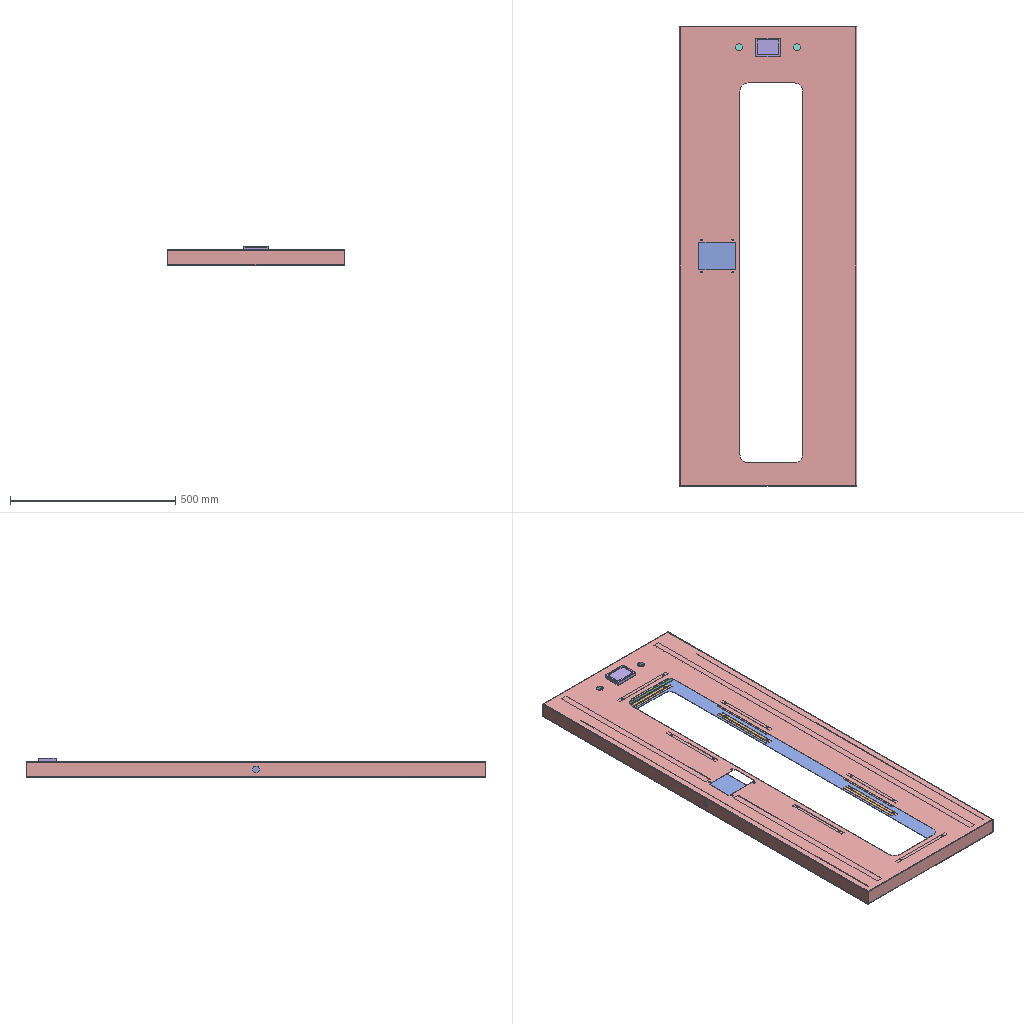Assembly | SolidWorks | 7 different items | 19 placed | box 536 x 1392 x 59 mm
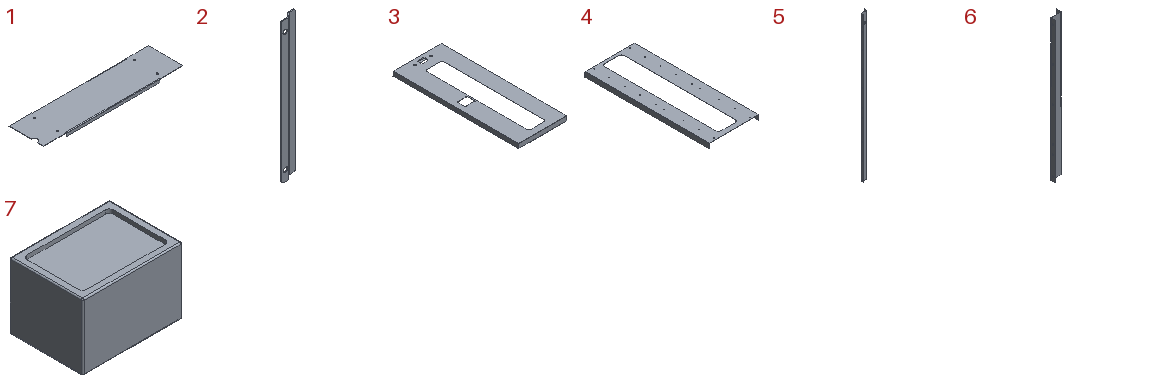Parts list (item | quantity | size | volume | features):
1 | x1 | 495 x 122 x 12 mm | 80038 mm3 | features Cut 2, EdgeFlange 2, FlatPattern 1, SMBaseFlange 1, SheetMetal 1
2 | x12 | 26 x 7.2 x 210 mm | 7055 mm3 | features BreakCorner 1, FlatPattern 1, ICE 1, SMBaseFlange 1, SheetMetal 1
3 | x1 | 536 x 1392 x 48.5 mm | 914346 mm3 | features ICE 3, EdgeFlange 2, CornerFeat 1, Cut 1, FlatPattern 1, SMBaseFlange 1, SheetMetal 1
4 | x1 | 495 x 1228 x 48 mm | 602812 mm3 | features Cut 3, EdgeFlange 1, FlatPattern 1, SMBaseFlange 1, SheetMetal 1
5 | x1 | 47.2 x 40 x 1350 mm | 135924 mm3 | features Cut 3, FlatPattern 1, SMBaseFlange 1, SheetMetal 1
6 | x2 | 47.2 x 40 x 615 mm | 62089 mm3 | features Cut 1, FlatPattern 1, SMBaseFlange 1, SheetMetal 1
7 | x1 | 75 x 55 x 50 mm | 197345 mm3 | features Fillet 2, Extrusion 1, ICE 1
Mates (type | each side: item.copy, entity, surface, feature):
Coincident | 3.1 face plane Base-Flange1 | 4.1 face plane Edge-Flange1
DistanceDim | 4.1 face plane Edge-Flange1 | 3.1 face plane Edge-Flange2 | 2 times
Coincident | 3.1 face plane Base-Flange1 | 5.1 face plane Base-Flange1
DistanceDim | 5.1 face plane Base-Flange1 | 3.1 face plane Edge-Flange2
DistanceDim | 5.1 face plane Base-Flange1 | 3.1 face plane Edge-Flange1
Coincident | 3.1 face plane Base-Flange1 | 6.1 face plane Base-Flange1
Parallel | 3.1 face plane Edge-Flange1 | 6.1 face plane Base-Flange1
DistanceDim | 6.1 face plane Base-Flange1 | 3.1 face plane Edge-Flange1
DistanceDim | 6.1 face plane Base-Flange1 | 3.1 face plane Edge-Flange2
Coincident | 4.1 face plane Base-Flange1 | 1.1 face plane Base-Flange1
DistanceDim | 1.1 face plane Edge-Flange2 | 3.1 face plane Edge-Flange2
DistanceDim | 1.1 face plane Base-Flange1 | 3.1 face plane Edge-Flange2
Coincident | 3.1 face plane Base-Flange1 | 2.1 face plane Base-Flange1
Width | 2.1 face plane Base-Flange1 | 2.1 face plane Base-Flange1 | 3.1 face plane Cut-Extrude1 | 3.1 face plane Cut-Extrude1
Coincident | 3.1 face plane Cut-Extrude1 | 2.1 face plane Base-Flange1
Coincident | 3.1 face plane Base-Flange1 | 2.2 face plane Base-Flange1
Coincident | 3.1 face plane Cut-Extrude1 | 2.2 face plane Base-Flange1
DistanceDim | 2.2 face plane Base-Flange1 | 3.1 face plane Cut-Extrude1
Coincident | 3.1 face plane Base-Flange1 | 2.3 face plane Base-Flange1
Coincident | 3.1 face plane Cut-Extrude1 | 2.3 face plane Base-Flange1
Coincident | 2.2 face plane Base-Flange1 | 2.3 face plane Base-Flange1
Coincident | 3.1 face plane Cut-Extrude1 | 7.1 face plane Boss-Extrude1 | 2 times
DistanceDim | 7.1 face plane Boss-Extrude1 | 3.1 face plane Base-Flange1